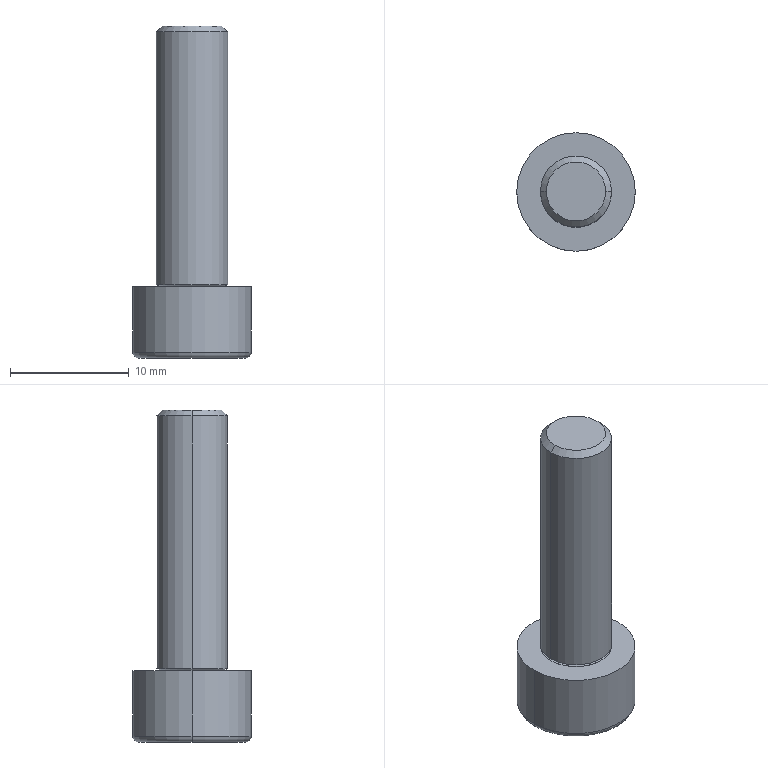Part | SolidWorks | features Attribute 1, Cut 1, Revolution 1 | 1 solid | 27 faces | box 10 x 10 x 28 mm | volume 1034 mm3 | plane 11 | torus 6 | cylinder 6 | cone 4 | commonest cylinder face diameters 6 x4 10 x2
STEP:
#1=CARTESIAN_POINT('',(-2.613,0.,0.01));
#2=VERTEX_POINT('',#1);
#3=CARTESIAN_POINT('',(-2.593,0.,0.03));
#4=VERTEX_POINT('',#3);
#5=CARTESIAN_POINT('',(-2.613,0.,0.03));
#6=DIRECTION('',(0.,-1.,0.));
#7=DIRECTION('',(0.,0.,-1.));
#8=AXIS2_PLACEMENT_3D('',#5,#6,#7);
#9=CIRCLE('',#8,0.02);
#10=EDGE_CURVE('',#2,#4,#9,.T.);
#11=ORIENTED_EDGE('',*,*,#10,.T.);
#12=CARTESIAN_POINT('',(2.593,0.,0.03));
#13=VERTEX_POINT('',#12);
#14=CARTESIAN_POINT('',(0.,0.,0.03));
#15=DIRECTION('',(0.,0.,-1.));
#16=DIRECTION('',(-1.,0.,0.));
#17=AXIS2_PLACEMENT_3D('',#14,#15,#16);
#18=CIRCLE('',#17,2.593);
#19=EDGE_CURVE('',#4,#13,#18,.T.);
#20=ORIENTED_EDGE('',*,*,#19,.T.);
#21=CARTESIAN_POINT('',(2.613,0.,0.01));
#22=VERTEX_POINT('',#21);
#23=CARTESIAN_POINT('',(2.613,0.,0.03));
#24=DIRECTION('',(0.,1.,0.));
#25=DIRECTION('',(-1.,0.,0.));
#26=AXIS2_PLACEMENT_3D('',#23,#24,#25);
#27=CIRCLE('',#26,0.02);
#28=EDGE_CURVE('',#22,#13,#27,.T.);
#29=ORIENTED_EDGE('',*,*,#28,.F.);
#30=CARTESIAN_POINT('',(0.,0.,0.01));
#31=DIRECTION('',(0.,0.,-1.));
#32=DIRECTION('',(-1.,0.,0.));
#33=AXIS2_PLACEMENT_3D('',#30,#31,#32);
#34=CIRCLE('',#33,2.613);
#35=EDGE_CURVE('',#2,#22,#34,.T.);
#36=ORIENTED_EDGE('',*,*,#35,.F.);
#37=EDGE_LOOP('',(#11,#20,#29,#36));
#38=FACE_OUTER_BOUND('',#37,.T.);
#39=CARTESIAN_POINT('',(0.,0.,0.03));
#40=DIRECTION('',(0.,0.,-1.));
#41=DIRECTION('',(-1.,0.,0.));
#42=AXIS2_PLACEMENT_3D('',#39,#40,#41);
#43=TOROIDAL_SURFACE('',#42,2.613,0.02);
#44=ADVANCED_FACE('',(#38),#43,.F.);
#45=ORIENTED_EDGE('',*,*,#28,.T.);
#46=CARTESIAN_POINT('',(0.,0.,0.03));
#47=DIRECTION('',(0.,0.,-1.));
#48=DIRECTION('',(-1.,0.,0.));
#49=AXIS2_PLACEMENT_3D('',#46,#47,#48);
#50=CIRCLE('',#49,2.593);
#51=EDGE_CURVE('',#13,#4,#50,.T.);
#52=ORIENTED_EDGE('',*,*,#51,.T.);
#53=ORIENTED_EDGE('',*,*,#10,.F.);
#54=CARTESIAN_POINT('',(0.,0.,0.01));
#55=DIRECTION('',(0.,0.,-1.));
#56=DIRECTION('',(-1.,0.,0.));
#57=AXIS2_PLACEMENT_3D('',#54,#55,#56);
#58=CIRCLE('',#57,2.613);
#59=EDGE_CURVE('',#22,#2,#58,.T.);
#60=ORIENTED_EDGE('',*,*,#59,.F.);
#61=EDGE_LOOP('',(#45,#52,#53,#60));
#62=FACE_OUTER_BOUND('',#61,.T.);
#63=CARTESIAN_POINT('',(0.,0.,0.03));
#64=DIRECTION('',(0.,0.,-1.));
#65=DIRECTION('',(-1.,0.,0.));
#66=AXIS2_PLACEMENT_3D('',#63,#64,#65);
#67=TOROIDAL_SURFACE('',#66,2.613,0.02);
#68=ADVANCED_FACE('',(#62),#67,.F.);
#69=CARTESIAN_POINT('',(-2.5,0.,22.));
#70=VERTEX_POINT('',#69);
#71=CARTESIAN_POINT('',(2.5,0.,22.));
#72=VERTEX_POINT('',#71);
#73=CARTESIAN_POINT('',(0.,0.,22.));
#74=DIRECTION('',(0.,0.,-1.));
#75=DIRECTION('',(-1.,0.,0.));
#76=AXIS2_PLACEMENT_3D('',#73,#74,#75);
#77=CIRCLE('',#76,2.5);
#78=EDGE_CURVE('',#70,#72,#77,.T.);
#79=ORIENTED_EDGE('',*,*,#78,.T.);
#80=CARTESIAN_POINT('',(3.,0.,21.5));
#81=VERTEX_POINT('',#80);
#82=CARTESIAN_POINT('',(2.5,0.,22.));
#83=DIRECTION('',(0.7071,0.,-0.7071));
#84=VECTOR('',#83,1000.);
#85=LINE('',#82,#84);
#86=EDGE_CURVE('',#72,#81,#85,.T.);
#87=ORIENTED_EDGE('',*,*,#86,.T.);
#88=CARTESIAN_POINT('',(-3.,0.,21.5));
#89=VERTEX_POINT('',#88);
#90=CARTESIAN_POINT('',(0.,0.,21.5));
#91=DIRECTION('',(0.,0.,-1.));
#92=DIRECTION('',(-1.,0.,0.));
#93=AXIS2_PLACEMENT_3D('',#90,#91,#92);
#94=CIRCLE('',#93,3.);
#95=EDGE_CURVE('',#89,#81,#94,.T.);
#96=ORIENTED_EDGE('',*,*,#95,.F.);
#97=CARTESIAN_POINT('',(-2.5,0.,22.));
#98=DIRECTION('',(-0.7071,0.,-0.7071));
#99=VECTOR('',#98,1000.);
#100=LINE('',#97,#99);
#101=EDGE_CURVE('',#70,#89,#100,.T.);
#102=ORIENTED_EDGE('',*,*,#101,.F.);
#103=EDGE_LOOP('',(#79,#87,#96,#102));
#104=FACE_OUTER_BOUND('',#103,.T.);
#105=CARTESIAN_POINT('',(0.,0.,22.));
#106=DIRECTION('',(0.,0.,-1.));
#107=DIRECTION('',(-1.,0.,0.));
#108=AXIS2_PLACEMENT_3D('',#105,#106,#107);
#109=CONICAL_SURFACE('',#108,2.5,0.7854);
#110=ADVANCED_FACE('',(#104),#109,.T.);
#111=ORIENTED_EDGE('',*,*,#95,.T.);
#112=CARTESIAN_POINT('',(3.,0.,0.192));
#113=VERTEX_POINT('',#112);
#114=CARTESIAN_POINT('',(3.,0.,-10.585));
#115=DIRECTION('',(0.,0.,-1.));
#116=VECTOR('',#115,1000.);
#117=LINE('',#114,#116);
#118=EDGE_CURVE('',#81,#113,#117,.T.);
#119=ORIENTED_EDGE('',*,*,#118,.T.);
#120=CARTESIAN_POINT('',(-3.,0.,0.192));
#121=VERTEX_POINT('',#120);
#122=CARTESIAN_POINT('',(0.,0.,0.192));
#123=DIRECTION('',(0.,0.,-1.));
#124=DIRECTION('',(-1.,0.,0.));
#125=AXIS2_PLACEMENT_3D('',#122,#123,#124);
#126=CIRCLE('',#125,3.);
#127=EDGE_CURVE('',#121,#113,#126,.T.);
#128=ORIENTED_EDGE('',*,*,#127,.F.);
#129=CARTESIAN_POINT('',(-3.,0.,-10.585));
#130=DIRECTION('',(0.,0.,-1.));
#131=VECTOR('',#130,1000.);
#132=LINE('',#129,#131);
#133=EDGE_CURVE('',#89,#121,#132,.T.);
#134=ORIENTED_EDGE('',*,*,#133,.F.);
#135=EDGE_LOOP('',(#111,#119,#128,#134));
#136=FACE_OUTER_BOUND('',#135,.T.);
#137=CARTESIAN_POINT('',(0.,0.,-10.585));
#138=DIRECTION('',(0.,0.,-1.));
#139=DIRECTION('',(-1.,0.,0.));
#140=AXIS2_PLACEMENT_3D('',#137,#138,#139);
#141=CYLINDRICAL_SURFACE('',#140,3.);
#142=ADVANCED_FACE('',(#136),#141,.T.);
#143=CARTESIAN_POINT('',(-2.607,0.,0.04879));
#144=VERTEX_POINT('',#143);
#145=CARTESIAN_POINT('',(2.607,0.,0.04879));
#146=VERTEX_POINT('',#145);
#147=CARTESIAN_POINT('',(0.,0.,0.04879));
#148=DIRECTION('',(0.,0.,-1.));
#149=DIRECTION('',(-1.,0.,0.));
#150=AXIS2_PLACEMENT_3D('',#147,#148,#149);
#151=CIRCLE('',#150,2.607);
#152=EDGE_CURVE('',#144,#146,#151,.T.);
#153=ORIENTED_EDGE('',*,*,#152,.F.);
#154=CARTESIAN_POINT('',(-3.,0.,0.192));
#155=DIRECTION('',(-0.9397,0.,0.342));
#156=VECTOR('',#155,1000.);
#157=LINE('',#154,#156);
#158=EDGE_CURVE('',#144,#121,#157,.T.);
#159=ORIENTED_EDGE('',*,*,#158,.T.);
#160=ORIENTED_EDGE('',*,*,#127,.T.);
#161=CARTESIAN_POINT('',(3.,0.,0.192));
#162=DIRECTION('',(0.9397,0.,0.342));
#163=VECTOR('',#162,1000.);
#164=LINE('',#161,#163);
#165=EDGE_CURVE('',#146,#113,#164,.T.);
#166=ORIENTED_EDGE('',*,*,#165,.F.);
#167=EDGE_LOOP('',(#153,#159,#160,#166));
#168=FACE_OUTER_BOUND('',#167,.T.);
#169=CARTESIAN_POINT('',(0.,0.,0.192));
#170=DIRECTION('',(0.,0.,1.));
#171=DIRECTION('',(1.,0.,0.));
#172=AXIS2_PLACEMENT_3D('',#169,#170,#171);
#173=CONICAL_SURFACE('',#172,3.,1.222);
#174=ADVANCED_FACE('',(#168),#173,.T.);
#175=ORIENTED_EDGE('',*,*,#51,.F.);
#176=CARTESIAN_POINT('',(2.613,0.,0.03));
#177=DIRECTION('',(0.,1.,0.));
#178=DIRECTION('',(-1.,0.,0.));
#179=AXIS2_PLACEMENT_3D('',#176,#177,#178);
#180=CIRCLE('',#179,0.02);
#181=EDGE_CURVE('',#13,#146,#180,.T.);
#182=ORIENTED_EDGE('',*,*,#181,.T.);
#183=CARTESIAN_POINT('',(0.,0.,0.04879));
#184=DIRECTION('',(0.,0.,-1.));
#185=DIRECTION('',(-1.,0.,0.));
#186=AXIS2_PLACEMENT_3D('',#183,#184,#185);
#187=CIRCLE('',#186,2.607);
#188=EDGE_CURVE('',#146,#144,#187,.T.);
#189=ORIENTED_EDGE('',*,*,#188,.T.);
#190=CARTESIAN_POINT('',(-2.613,0.,0.03));
#191=DIRECTION('',(0.,-1.,0.));
#192=DIRECTION('',(0.,0.,-1.));
#193=AXIS2_PLACEMENT_3D('',#190,#191,#192);
#194=CIRCLE('',#193,0.02);
#195=EDGE_CURVE('',#4,#144,#194,.T.);
#196=ORIENTED_EDGE('',*,*,#195,.F.);
#197=EDGE_LOOP('',(#175,#182,#189,#196));
#198=FACE_OUTER_BOUND('',#197,.T.);
#199=CARTESIAN_POINT('',(0.,0.,0.03));
#200=DIRECTION('',(0.,0.,-1.));
#201=DIRECTION('',(-1.,0.,0.));
#202=AXIS2_PLACEMENT_3D('',#199,#200,#201);
#203=TOROIDAL_SURFACE('',#202,2.613,0.02);
#204=ADVANCED_FACE('',(#198),#203,.F.);
#205=CARTESIAN_POINT('',(-3.,0.,0.01));
#206=VERTEX_POINT('',#205);
#207=CARTESIAN_POINT('',(3.,0.,0.01));
#208=VERTEX_POINT('',#207);
#209=CARTESIAN_POINT('',(0.,0.,0.01));
#210=DIRECTION('',(0.,0.,-1.));
#211=DIRECTION('',(-1.,0.,0.));
#212=AXIS2_PLACEMENT_3D('',#209,#210,#211);
#213=CIRCLE('',#212,3.);
#214=EDGE_CURVE('',#206,#208,#213,.T.);
#215=ORIENTED_EDGE('',*,*,#214,.T.);
#216=CARTESIAN_POINT('',(3.,0.,0.));
#217=VERTEX_POINT('',#216);
#218=CARTESIAN_POINT('',(3.,0.,-10.585));
#219=DIRECTION('',(0.,0.,-1.));
#220=VECTOR('',#219,1000.);
#221=LINE('',#218,#220);
#222=EDGE_CURVE('',#208,#217,#221,.T.);
#223=ORIENTED_EDGE('',*,*,#222,.T.);
#224=CARTESIAN_POINT('',(-3.,0.,0.));
#225=VERTEX_POINT('',#224);
#226=CARTESIAN_POINT('',(0.,0.,0.));
#227=DIRECTION('',(0.,0.,-1.));
#228=DIRECTION('',(-1.,0.,0.));
#229=AXIS2_PLACEMENT_3D('',#226,#227,#228);
#230=CIRCLE('',#229,3.);
#231=EDGE_CURVE('',#225,#217,#230,.T.);
#232=ORIENTED_EDGE('',*,*,#231,.F.);
#233=CARTESIAN_POINT('',(-3.,0.,-10.585));
#234=DIRECTION('',(0.,0.,-1.));
#235=VECTOR('',#234,1000.);
#236=LINE('',#233,#235);
#237=EDGE_CURVE('',#206,#225,#236,.T.);
#238=ORIENTED_EDGE('',*,*,#237,.F.);
#239=EDGE_LOOP('',(#215,#223,#232,#238));
#240=FACE_OUTER_BOUND('',#239,.T.);
#241=CARTESIAN_POINT('',(0.,0.,-10.585));
#242=DIRECTION('',(0.,0.,-1.));
#243=DIRECTION('',(-1.,0.,0.));
#244=AXIS2_PLACEMENT_3D('',#241,#242,#243);
#245=CYLINDRICAL_SURFACE('',#244,3.);
#246=ADVANCED_FACE('',(#240),#245,.T.);
#247=CARTESIAN_POINT('',(-5.,0.,0.));
#248=VERTEX_POINT('',#247);
#249=CARTESIAN_POINT('',(5.,0.,0.));
#250=VERTEX_POINT('',#249);
#251=CARTESIAN_POINT('',(0.,0.,0.));
#252=DIRECTION('',(0.,0.,-1.));
#253=DIRECTION('',(-1.,0.,0.));
#254=AXIS2_PLACEMENT_3D('',#251,#252,#253);
#255=CIRCLE('',#254,5.);
#256=EDGE_CURVE('',#248,#250,#255,.T.);
#257=ORIENTED_EDGE('',*,*,#256,.T.);
#258=CARTESIAN_POINT('',(5.,0.,-5.5));
#259=VERTEX_POINT('',#258);
#260=CARTESIAN_POINT('',(5.,0.,-10.585));
#261=DIRECTION('',(0.,0.,-1.));
#262=VECTOR('',#261,1000.);
#263=LINE('',#260,#262);
#264=EDGE_CURVE('',#250,#259,#263,.T.);
#265=ORIENTED_EDGE('',*,*,#264,.T.);
#266=CARTESIAN_POINT('',(-5.,0.,-5.5));
#267=VERTEX_POINT('',#266);
#268=CARTESIAN_POINT('',(0.,0.,-5.5));
#269=DIRECTION('',(0.,0.,-1.));
#270=DIRECTION('',(-1.,0.,0.));
#271=AXIS2_PLACEMENT_3D('',#268,#269,#270);
#272=CIRCLE('',#271,5.);
#273=EDGE_CURVE('',#267,#259,#272,.T.);
#274=ORIENTED_EDGE('',*,*,#273,.F.);
#275=CARTESIAN_POINT('',(-5.,0.,-10.585));
#276=DIRECTION('',(0.,0.,-1.));
#277=VECTOR('',#276,1000.);
#278=LINE('',#275,#277);
#279=EDGE_CURVE('',#248,#267,#278,.T.);
#280=ORIENTED_EDGE('',*,*,#279,.F.);
#281=EDGE_LOOP('',(#257,#265,#274,#280));
#282=FACE_OUTER_BOUND('',#281,.T.);
#283=CARTESIAN_POINT('',(0.,0.,-10.585));
#284=DIRECTION('',(0.,0.,-1.));
#285=DIRECTION('',(-1.,0.,0.));
#286=AXIS2_PLACEMENT_3D('',#283,#284,#285);
#287=CYLINDRICAL_SURFACE('',#286,5.);
#288=ADVANCED_FACE('',(#282),#287,.T.);
#289=ORIENTED_EDGE('',*,*,#273,.T.);
#290=CARTESIAN_POINT('',(4.5,0.,-6.));
#291=VERTEX_POINT('',#290);
#292=CARTESIAN_POINT('',(4.5,0.,-5.5));
#293=DIRECTION('',(0.,1.,0.));
#294=DIRECTION('',(-1.,0.,0.));
#295=AXIS2_PLACEMENT_3D('',#292,#293,#294);
#296=CIRCLE('',#295,0.5);
#297=EDGE_CURVE('',#259,#291,#296,.T.);
#298=ORIENTED_EDGE('',*,*,#297,.T.);
#299=CARTESIAN_POINT('',(-4.5,0.,-6.));
#300=VERTEX_POINT('',#299);
#301=CARTESIAN_POINT('',(0.,0.,-6.));
#302=DIRECTION('',(0.,0.,-1.));
#303=DIRECTION('',(-1.,0.,0.));
#304=AXIS2_PLACEMENT_3D('',#301,#302,#303);
#305=CIRCLE('',#304,4.5);
#306=EDGE_CURVE('',#300,#291,#305,.T.);
#307=ORIENTED_EDGE('',*,*,#306,.F.);
#308=CARTESIAN_POINT('',(-4.5,0.,-5.5));
#309=DIRECTION('',(0.,-1.,0.));
#310=DIRECTION('',(0.,0.,-1.));
#311=AXIS2_PLACEMENT_3D('',#308,#309,#310);
#312=CIRCLE('',#311,0.5);
#313=EDGE_CURVE('',#267,#300,#312,.T.);
#314=ORIENTED_EDGE('',*,*,#313,.F.);
#315=EDGE_LOOP('',(#289,#298,#307,#314));
#316=FACE_OUTER_BOUND('',#315,.T.);
#317=CARTESIAN_POINT('',(0.,0.,-5.5));
#318=DIRECTION('',(0.,0.,-1.));
#319=DIRECTION('',(-1.,0.,0.));
#320=AXIS2_PLACEMENT_3D('',#317,#318,#319);
#321=TOROIDAL_SURFACE('',#320,4.5,0.5);
#322=ADVANCED_FACE('',(#316),#321,.T.);
#323=ORIENTED_EDGE('',*,*,#297,.F.);
#324=CARTESIAN_POINT('',(0.,0.,-5.5));
#325=DIRECTION('',(0.,0.,-1.));
#326=DIRECTION('',(-1.,0.,0.));
#327=AXIS2_PLACEMENT_3D('',#324,#325,#326);
#328=CIRCLE('',#327,5.);
#329=EDGE_CURVE('',#259,#267,#328,.T.);
#330=ORIENTED_EDGE('',*,*,#329,.T.);
#331=ORIENTED_EDGE('',*,*,#313,.T.);
#332=CARTESIAN_POINT('',(0.,0.,-6.));
#333=DIRECTION('',(0.,0.,-1.));
#334=DIRECTION('',(-1.,0.,0.));
#335=AXIS2_PLACEMENT_3D('',#332,#333,#334);
#336=CIRCLE('',#335,4.5);
#337=EDGE_CURVE('',#291,#300,#336,.T.);
#338=ORIENTED_EDGE('',*,*,#337,.F.);
#339=EDGE_LOOP('',(#323,#330,#331,#338));
#340=FACE_OUTER_BOUND('',#339,.T.);
#341=CARTESIAN_POINT('',(0.,0.,-5.5));
#342=DIRECTION('',(0.,0.,-1.));
#343=DIRECTION('',(-1.,0.,0.));
#344=AXIS2_PLACEMENT_3D('',#341,#342,#343);
#345=TOROIDAL_SURFACE('',#344,4.5,0.5);
#346=ADVANCED_FACE('',(#340),#345,.T.);
#347=ORIENTED_EDGE('',*,*,#264,.F.);
#348=CARTESIAN_POINT('',(0.,0.,0.));
#349=DIRECTION('',(0.,0.,-1.));
#350=DIRECTION('',(-1.,0.,0.));
#351=AXIS2_PLACEMENT_3D('',#348,#349,#350);
#352=CIRCLE('',#351,5.);
#353=EDGE_CURVE('',#250,#248,#352,.T.);
#354=ORIENTED_EDGE('',*,*,#353,.T.);
#355=ORIENTED_EDGE('',*,*,#279,.T.);
#356=ORIENTED_EDGE('',*,*,#329,.F.);
#357=EDGE_LOOP('',(#347,#354,#355,#356));
#358=FACE_OUTER_BOUND('',#357,.T.);
#359=CARTESIAN_POINT('',(0.,0.,-10.585));
#360=DIRECTION('',(0.,0.,-1.));
#361=DIRECTION('',(-1.,0.,0.));
#362=AXIS2_PLACEMENT_3D('',#359,#360,#361);
#363=CYLINDRICAL_SURFACE('',#362,5.);
#364=ADVANCED_FACE('',(#358),#363,.T.);
#365=ORIENTED_EDGE('',*,*,#256,.F.);
#366=ORIENTED_EDGE('',*,*,#353,.F.);
#367=EDGE_LOOP('',(#365,#366));
#368=FACE_OUTER_BOUND('',#367,.T.);
#369=ORIENTED_EDGE('',*,*,#231,.T.);
#370=CARTESIAN_POINT('',(0.,0.,0.));
#371=DIRECTION('',(0.,0.,-1.));
#372=DIRECTION('',(-1.,0.,0.));
#373=AXIS2_PLACEMENT_3D('',#370,#371,#372);
#374=CIRCLE('',#373,3.);
#375=EDGE_CURVE('',#217,#225,#374,.T.);
#376=ORIENTED_EDGE('',*,*,#375,.T.);
#377=EDGE_LOOP('',(#369,#376));
#378=FACE_BOUND('',#377,.T.);
#379=CARTESIAN_POINT('',(-5.,0.,0.));
#380=DIRECTION('',(0.,0.,-1.));
#381=DIRECTION('',(-1.,0.,0.));
#382=AXIS2_PLACEMENT_3D('',#379,#380,#381);
#383=PLANE('',#382);
#384=ADVANCED_FACE('',(#368,#378),#383,.F.);
#385=ORIENTED_EDGE('',*,*,#222,.F.);
#386=CARTESIAN_POINT('',(0.,0.,0.01));
#387=DIRECTION('',(0.,0.,-1.));
#388=DIRECTION('',(-1.,0.,0.));
#389=AXIS2_PLACEMENT_3D('',#386,#387,#388);
#390=CIRCLE('',#389,3.);
#391=EDGE_CURVE('',#208,#206,#390,.T.);
#392=ORIENTED_EDGE('',*,*,#391,.T.);
#393=ORIENTED_EDGE('',*,*,#237,.T.);
#394=ORIENTED_EDGE('',*,*,#375,.F.);
#395=EDGE_LOOP('',(#385,#392,#393,#394));
#396=FACE_OUTER_BOUND('',#395,.T.);
#397=CARTESIAN_POINT('',(0.,0.,-10.585));
#398=DIRECTION('',(0.,0.,-1.));
#399=DIRECTION('',(-1.,0.,0.));
#400=AXIS2_PLACEMENT_3D('',#397,#398,#399);
#401=CYLINDRICAL_SURFACE('',#400,3.);
#402=ADVANCED_FACE('',(#396),#401,.T.);
#403=ORIENTED_EDGE('',*,*,#214,.F.);
#404=ORIENTED_EDGE('',*,*,#391,.F.);
#405=EDGE_LOOP('',(#403,#404));
#406=FACE_OUTER_BOUND('',#405,.T.);
#407=ORIENTED_EDGE('',*,*,#35,.T.);
#408=ORIENTED_EDGE('',*,*,#59,.T.);
#409=EDGE_LOOP('',(#407,#408));
#410=FACE_BOUND('',#409,.T.);
#411=CARTESIAN_POINT('',(-3.,0.,0.01));
#412=DIRECTION('',(0.,0.,-1.));
#413=DIRECTION('',(-1.,0.,0.));
#414=AXIS2_PLACEMENT_3D('',#411,#412,#413);
#415=PLANE('',#414);
#416=ADVANCED_FACE('',(#406,#410),#415,.F.);
#417=ORIENTED_EDGE('',*,*,#19,.F.);
#418=ORIENTED_EDGE('',*,*,#195,.T.);
#419=ORIENTED_EDGE('',*,*,#152,.T.);
#420=ORIENTED_EDGE('',*,*,#181,.F.);
#421=EDGE_LOOP('',(#417,#418,#419,#420));
#422=FACE_OUTER_BOUND('',#421,.T.);
#423=CARTESIAN_POINT('',(0.,0.,0.03));
#424=DIRECTION('',(0.,0.,-1.));
#425=DIRECTION('',(-1.,0.,0.));
#426=AXIS2_PLACEMENT_3D('',#423,#424,#425);
#427=TOROIDAL_SURFACE('',#426,2.613,0.02);
#428=ADVANCED_FACE('',(#422),#427,.F.);
#429=ORIENTED_EDGE('',*,*,#158,.F.);
#430=ORIENTED_EDGE('',*,*,#188,.F.);
#431=ORIENTED_EDGE('',*,*,#165,.T.);
#432=CARTESIAN_POINT('',(0.,0.,0.192));
#433=DIRECTION('',(0.,0.,-1.));
#434=DIRECTION('',(-1.,0.,0.));
#435=AXIS2_PLACEMENT_3D('',#432,#433,#434);
#436=CIRCLE('',#435,3.);
#437=EDGE_CURVE('',#113,#121,#436,.T.);
#438=ORIENTED_EDGE('',*,*,#437,.T.);
#439=EDGE_LOOP('',(#429,#430,#431,#438));
#440=FACE_OUTER_BOUND('',#439,.T.);
#441=CARTESIAN_POINT('',(0.,0.,0.192));
#442=DIRECTION('',(0.,0.,1.));
#443=DIRECTION('',(1.,0.,0.));
#444=AXIS2_PLACEMENT_3D('',#441,#442,#443);
#445=CONICAL_SURFACE('',#444,3.,1.222);
#446=ADVANCED_FACE('',(#440),#445,.T.);
#447=ORIENTED_EDGE('',*,*,#118,.F.);
#448=CARTESIAN_POINT('',(0.,0.,21.5));
#449=DIRECTION('',(0.,0.,-1.));
#450=DIRECTION('',(-1.,0.,0.));
#451=AXIS2_PLACEMENT_3D('',#448,#449,#450);
#452=CIRCLE('',#451,3.);
#453=EDGE_CURVE('',#81,#89,#452,.T.);
#454=ORIENTED_EDGE('',*,*,#453,.T.);
#455=ORIENTED_EDGE('',*,*,#133,.T.);
#456=ORIENTED_EDGE('',*,*,#437,.F.);
#457=EDGE_LOOP('',(#447,#454,#455,#456));
#458=FACE_OUTER_BOUND('',#457,.T.);
#459=CARTESIAN_POINT('',(0.,0.,-10.585));
#460=DIRECTION('',(0.,0.,-1.));
#461=DIRECTION('',(-1.,0.,0.));
#462=AXIS2_PLACEMENT_3D('',#459,#460,#461);
#463=CYLINDRICAL_SURFACE('',#462,3.);
#464=ADVANCED_FACE('',(#458),#463,.T.);
#465=ORIENTED_EDGE('',*,*,#86,.F.);
#466=CARTESIAN_POINT('',(0.,0.,22.));
#467=DIRECTION('',(0.,0.,-1.));
#468=DIRECTION('',(-1.,0.,0.));
#469=AXIS2_PLACEMENT_3D('',#466,#467,#468);
#470=CIRCLE('',#469,2.5);
#471=EDGE_CURVE('',#72,#70,#470,.T.);
#472=ORIENTED_EDGE('',*,*,#471,.T.);
#473=ORIENTED_EDGE('',*,*,#101,.T.);
#474=ORIENTED_EDGE('',*,*,#453,.F.);
#475=EDGE_LOOP('',(#465,#472,#473,#474));
#476=FACE_OUTER_BOUND('',#475,.T.);
#477=CARTESIAN_POINT('',(0.,0.,22.));
#478=DIRECTION('',(0.,0.,-1.));
#479=DIRECTION('',(-1.,0.,0.));
#480=AXIS2_PLACEMENT_3D('',#477,#478,#479);
#481=CONICAL_SURFACE('',#480,2.5,0.7854);
#482=ADVANCED_FACE('',(#476),#481,.T.);
#483=ORIENTED_EDGE('',*,*,#78,.F.);
#484=ORIENTED_EDGE('',*,*,#471,.F.);
#485=EDGE_LOOP('',(#483,#484));
#486=FACE_OUTER_BOUND('',#485,.T.);
#487=CARTESIAN_POINT('',(-2.5,0.,22.));
#488=DIRECTION('',(0.,0.,-1.));
#489=DIRECTION('',(-1.,0.,0.));
#490=AXIS2_PLACEMENT_3D('',#487,#488,#489);
#491=PLANE('',#490);
#492=ADVANCED_FACE('',(#486),#491,.F.);
#493=CARTESIAN_POINT('',(2.887,0.,-6.));
#494=VERTEX_POINT('',#493);
#495=CARTESIAN_POINT('',(1.443,-2.5,-6.));
#496=VERTEX_POINT('',#495);
#497=CARTESIAN_POINT('',(2.887,0.,-6.));
#498=DIRECTION('',(-0.5,-0.866,0.));
#499=VECTOR('',#498,1000.);
#500=LINE('',#497,#499);
#501=EDGE_CURVE('',#494,#496,#500,.T.);
#502=ORIENTED_EDGE('',*,*,#501,.F.);
#503=CARTESIAN_POINT('',(1.443,2.5,-6.));
#504=VERTEX_POINT('',#503);
#505=CARTESIAN_POINT('',(1.443,2.5,-6.));
#506=DIRECTION('',(0.5,-0.866,0.));
#507=VECTOR('',#506,1000.);
#508=LINE('',#505,#507);
#509=EDGE_CURVE('',#504,#494,#508,.T.);
#510=ORIENTED_EDGE('',*,*,#509,.F.);
#511=CARTESIAN_POINT('',(-1.443,2.5,-6.));
#512=VERTEX_POINT('',#511);
#513=CARTESIAN_POINT('',(-1.443,2.5,-6.));
#514=DIRECTION('',(1.,0.,0.));
#515=VECTOR('',#514,1000.);
#516=LINE('',#513,#515);
#517=EDGE_CURVE('',#512,#504,#516,.T.);
#518=ORIENTED_EDGE('',*,*,#517,.F.);
#519=CARTESIAN_POINT('',(-2.887,0.,-6.));
#520=VERTEX_POINT('',#519);
#521=CARTESIAN_POINT('',(-2.887,0.,-6.));
#522=DIRECTION('',(0.5,0.866,0.));
#523=VECTOR('',#522,1000.);
#524=LINE('',#521,#523);
#525=EDGE_CURVE('',#520,#512,#524,.T.);
#526=ORIENTED_EDGE('',*,*,#525,.F.);
#527=CARTESIAN_POINT('',(-1.443,-2.5,-6.));
#528=VERTEX_POINT('',#527);
#529=CARTESIAN_POINT('',(-1.443,-2.5,-6.));
#530=DIRECTION('',(-0.5,0.866,0.));
#531=VECTOR('',#530,1000.);
#532=LINE('',#529,#531);
#533=EDGE_CURVE('',#528,#520,#532,.T.);
#534=ORIENTED_EDGE('',*,*,#533,.F.);
#535=CARTESIAN_POINT('',(1.443,-2.5,-6.));
#536=DIRECTION('',(-1.,0.,0.));
#537=VECTOR('',#536,1000.);
#538=LINE('',#535,#537);
#539=EDGE_CURVE('',#496,#528,#538,.T.);
#540=ORIENTED_EDGE('',*,*,#539,.F.);
#541=EDGE_LOOP('',(#502,#510,#518,#526,#534,#540));
#542=FACE_BOUND('',#541,.T.);
#543=ORIENTED_EDGE('',*,*,#306,.T.);
#544=ORIENTED_EDGE('',*,*,#337,.T.);
#545=EDGE_LOOP('',(#543,#544));
#546=FACE_OUTER_BOUND('',#545,.T.);
#547=CARTESIAN_POINT('',(0.,0.,-6.));
#548=DIRECTION('',(0.,0.,1.));
#549=DIRECTION('',(1.,0.,0.));
#550=AXIS2_PLACEMENT_3D('',#547,#548,#549);
#551=PLANE('',#550);
#552=ADVANCED_FACE('',(#542,#546),#551,.F.);
#553=ORIENTED_EDGE('',*,*,#509,.T.);
#554=CARTESIAN_POINT('',(2.887,0.,-3.5));
#555=VERTEX_POINT('',#554);
#556=CARTESIAN_POINT('',(2.887,0.,-3.5));
#557=DIRECTION('',(0.,0.,-1.));
#558=VECTOR('',#557,1000.);
#559=LINE('',#556,#558);
#560=EDGE_CURVE('',#555,#494,#559,.T.);
#561=ORIENTED_EDGE('',*,*,#560,.F.);
#562=CARTESIAN_POINT('',(1.443,2.5,-3.5));
#563=VERTEX_POINT('',#562);
#564=CARTESIAN_POINT('',(1.443,2.5,-3.5));
#565=DIRECTION('',(0.5,-0.866,0.));
#566=VECTOR('',#565,1000.);
#567=LINE('',#564,#566);
#568=EDGE_CURVE('',#563,#555,#567,.T.);
#569=ORIENTED_EDGE('',*,*,#568,.F.);
#570=CARTESIAN_POINT('',(1.443,2.5,-3.5));
#571=DIRECTION('',(0.,0.,-1.));
#572=VECTOR('',#571,1000.);
#573=LINE('',#570,#572);
#574=EDGE_CURVE('',#563,#504,#573,.T.);
#575=ORIENTED_EDGE('',*,*,#574,.T.);
#576=EDGE_LOOP('',(#553,#561,#569,#575));
#577=FACE_OUTER_BOUND('',#576,.T.);
#578=CARTESIAN_POINT('',(1.443,2.5,-3.5));
#579=DIRECTION('',(0.866,0.5,0.));
#580=DIRECTION('',(-0.5,0.866,0.));
#581=AXIS2_PLACEMENT_3D('',#578,#579,#580);
#582=PLANE('',#581);
#583=ADVANCED_FACE('',(#577),#582,.F.);
#584=ORIENTED_EDGE('',*,*,#517,.T.);
#585=ORIENTED_EDGE('',*,*,#574,.F.);
#586=CARTESIAN_POINT('',(-1.443,2.5,-3.5));
#587=VERTEX_POINT('',#586);
#588=CARTESIAN_POINT('',(-1.443,2.5,-3.5));
#589=DIRECTION('',(1.,0.,0.));
#590=VECTOR('',#589,1000.);
#591=LINE('',#588,#590);
#592=EDGE_CURVE('',#587,#563,#591,.T.);
#593=ORIENTED_EDGE('',*,*,#592,.F.);
#594=CARTESIAN_POINT('',(-1.443,2.5,-3.5));
#595=DIRECTION('',(0.,0.,-1.));
#596=VECTOR('',#595,1000.);
#597=LINE('',#594,#596);
#598=EDGE_CURVE('',#587,#512,#597,.T.);
#599=ORIENTED_EDGE('',*,*,#598,.T.);
#600=EDGE_LOOP('',(#584,#585,#593,#599));
#601=FACE_OUTER_BOUND('',#600,.T.);
#602=CARTESIAN_POINT('',(-1.443,2.5,-3.5));
#603=DIRECTION('',(0.,1.,0.));
#604=DIRECTION('',(-1.,0.,0.));
#605=AXIS2_PLACEMENT_3D('',#602,#603,#604);
#606=PLANE('',#605);
#607=ADVANCED_FACE('',(#601),#606,.F.);
#608=ORIENTED_EDGE('',*,*,#525,.T.);
#609=ORIENTED_EDGE('',*,*,#598,.F.);
#610=CARTESIAN_POINT('',(-2.887,0.,-3.5));
#611=VERTEX_POINT('',#610);
#612=CARTESIAN_POINT('',(-2.887,0.,-3.5));
#613=DIRECTION('',(0.5,0.866,0.));
#614=VECTOR('',#613,1000.);
#615=LINE('',#612,#614);
#616=EDGE_CURVE('',#611,#587,#615,.T.);
#617=ORIENTED_EDGE('',*,*,#616,.F.);
#618=CARTESIAN_POINT('',(-2.887,0.,-3.5));
#619=DIRECTION('',(0.,0.,-1.));
#620=VECTOR('',#619,1000.);
#621=LINE('',#618,#620);
#622=EDGE_CURVE('',#611,#520,#621,.T.);
#623=ORIENTED_EDGE('',*,*,#622,.T.);
#624=EDGE_LOOP('',(#608,#609,#617,#623));
#625=FACE_OUTER_BOUND('',#624,.T.);
#626=CARTESIAN_POINT('',(-2.887,0.,-3.5));
#627=DIRECTION('',(-0.866,0.5,0.));
#628=DIRECTION('',(-0.5,-0.866,0.));
#629=AXIS2_PLACEMENT_3D('',#626,#627,#628);
#630=PLANE('',#629);
#631=ADVANCED_FACE('',(#625),#630,.F.);
#632=ORIENTED_EDGE('',*,*,#533,.T.);
#633=ORIENTED_EDGE('',*,*,#622,.F.);
#634=CARTESIAN_POINT('',(-1.443,-2.5,-3.5));
#635=VERTEX_POINT('',#634);
#636=CARTESIAN_POINT('',(-1.443,-2.5,-3.5));
#637=DIRECTION('',(-0.5,0.866,0.));
#638=VECTOR('',#637,1000.);
#639=LINE('',#636,#638);
#640=EDGE_CURVE('',#635,#611,#639,.T.);
#641=ORIENTED_EDGE('',*,*,#640,.F.);
#642=CARTESIAN_POINT('',(-1.443,-2.5,-3.5));
#643=DIRECTION('',(0.,0.,-1.));
#644=VECTOR('',#643,1000.);
#645=LINE('',#642,#644);
#646=EDGE_CURVE('',#635,#528,#645,.T.);
#647=ORIENTED_EDGE('',*,*,#646,.T.);
#648=EDGE_LOOP('',(#632,#633,#641,#647));
#649=FACE_OUTER_BOUND('',#648,.T.);
#650=CARTESIAN_POINT('',(-1.443,-2.5,-3.5));
#651=DIRECTION('',(-0.866,-0.5,0.));
#652=DIRECTION('',(0.5,-0.866,0.));
#653=AXIS2_PLACEMENT_3D('',#650,#651,#652);
#654=PLANE('',#653);
#655=ADVANCED_FACE('',(#649),#654,.F.);
#656=ORIENTED_EDGE('',*,*,#539,.T.);
#657=ORIENTED_EDGE('',*,*,#646,.F.);
#658=CARTESIAN_POINT('',(1.443,-2.5,-3.5));
#659=VERTEX_POINT('',#658);
#660=CARTESIAN_POINT('',(1.443,-2.5,-3.5));
#661=DIRECTION('',(-1.,0.,0.));
#662=VECTOR('',#661,1000.);
#663=LINE('',#660,#662);
#664=EDGE_CURVE('',#659,#635,#663,.T.);
#665=ORIENTED_EDGE('',*,*,#664,.F.);
#666=CARTESIAN_POINT('',(1.443,-2.5,-3.5));
#667=DIRECTION('',(0.,0.,-1.));
#668=VECTOR('',#667,1000.);
#669=LINE('',#666,#668);
#670=EDGE_CURVE('',#659,#496,#669,.T.);
#671=ORIENTED_EDGE('',*,*,#670,.T.);
#672=EDGE_LOOP('',(#656,#657,#665,#671));
#673=FACE_OUTER_BOUND('',#672,.T.);
#674=CARTESIAN_POINT('',(1.443,-2.5,-3.5));
#675=DIRECTION('',(0.,-1.,0.));
#676=DIRECTION('',(0.,0.,-1.));
#677=AXIS2_PLACEMENT_3D('',#674,#675,#676);
#678=PLANE('',#677);
#679=ADVANCED_FACE('',(#673),#678,.F.);
#680=ORIENTED_EDGE('',*,*,#501,.T.);
#681=ORIENTED_EDGE('',*,*,#670,.F.);
#682=CARTESIAN_POINT('',(2.887,0.,-3.5));
#683=DIRECTION('',(-0.5,-0.866,0.));
#684=VECTOR('',#683,1000.);
#685=LINE('',#682,#684);
#686=EDGE_CURVE('',#555,#659,#685,.T.);
#687=ORIENTED_EDGE('',*,*,#686,.F.);
#688=ORIENTED_EDGE('',*,*,#560,.T.);
#689=EDGE_LOOP('',(#680,#681,#687,#688));
#690=FACE_OUTER_BOUND('',#689,.T.);
#691=CARTESIAN_POINT('',(2.887,0.,-3.5));
#692=DIRECTION('',(0.866,-0.5,0.));
#693=DIRECTION('',(0.5,0.866,0.));
#694=AXIS2_PLACEMENT_3D('',#691,#692,#693);
#695=PLANE('',#694);
#696=ADVANCED_FACE('',(#690),#695,.F.);
#697=ORIENTED_EDGE('',*,*,#568,.T.);
#698=ORIENTED_EDGE('',*,*,#686,.T.);
#699=ORIENTED_EDGE('',*,*,#664,.T.);
#700=ORIENTED_EDGE('',*,*,#640,.T.);
#701=ORIENTED_EDGE('',*,*,#616,.T.);
#702=ORIENTED_EDGE('',*,*,#592,.T.);
#703=EDGE_LOOP('',(#697,#698,#699,#700,#701,#702));
#704=FACE_OUTER_BOUND('',#703,.T.);
#705=CARTESIAN_POINT('',(1.443,2.5,-3.5));
#706=DIRECTION('',(0.,0.,1.));
#707=DIRECTION('',(1.,0.,0.));
#708=AXIS2_PLACEMENT_3D('',#705,#706,#707);
#709=PLANE('',#708);
#710=ADVANCED_FACE('',(#704),#709,.F.);
#711=CLOSED_SHELL('',(#44,#68,#110,#142,#174,#204,#246,#288,#322,#346,#364,#384,#402,#416,#428,#446,#464,#482,#492,#552,#583,#607,#631,#655,#679,#696,#710));
#712=MANIFOLD_SOLID_BREP('',#711);
#713=CARTESIAN_POINT('',(0.,0.,0.));
#714=DIRECTION('',(0.,0.,1.));
#715=DIRECTION('',(1.,0.,0.));
#716=AXIS2_PLACEMENT_3D('',#713,#714,#715);
#717=(LENGTH_UNIT()NAMED_UNIT(*)SI_UNIT(.MILLI.,.METRE.));
#718=UNCERTAINTY_MEASURE_WITH_UNIT(LENGTH_MEASURE(0.00001),#717,'','');
#719=(NAMED_UNIT(*)PLANE_ANGLE_UNIT()SI_UNIT($,.RADIAN.));
#720=(NAMED_UNIT(*)SI_UNIT($,.STERADIAN.)SOLID_ANGLE_UNIT());
#721=(GEOMETRIC_REPRESENTATION_CONTEXT(3)GLOBAL_UNCERTAINTY_ASSIGNED_CONTEXT((#718))GLOBAL_UNIT_ASSIGNED_CONTEXT((#717,#719,#720))REPRESENTATION_CONTEXT('',''));
#722=ADVANCED_BREP_SHAPE_REPRESENTATION('',(#712,#716),#721);